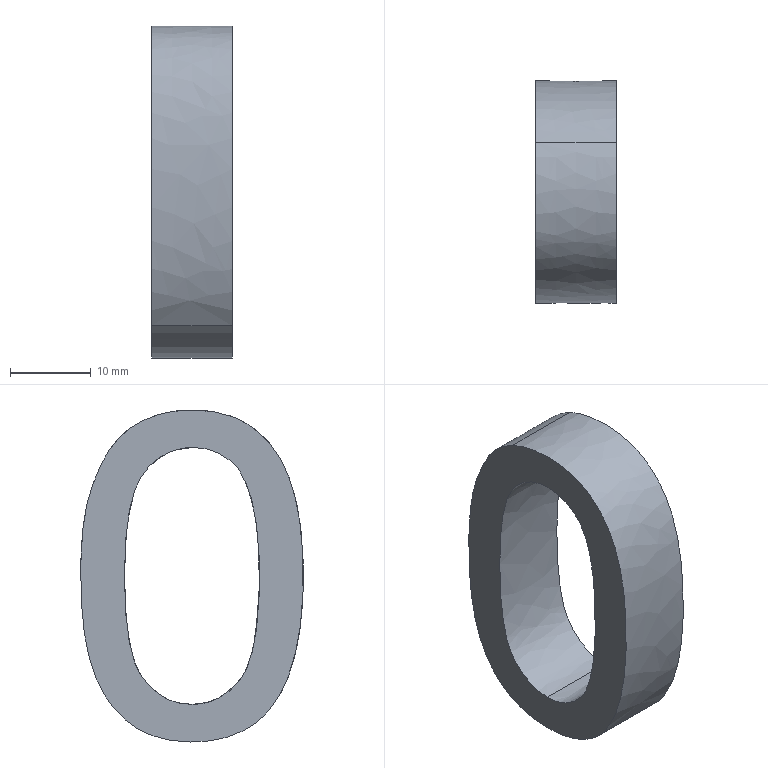Part | NX | features solid 2 | 1 solid | 7 faces | box 10 x 27.595 x 41.147 mm | volume 5024 mm3 | spline 5 | plane 2
STEP:
#1=CARTESIAN_POINT('',(2250.,-393.803,-666.115));
#2=VERTEX_POINT('',#1);
#3=CARTESIAN_POINT('',(2250.,-393.879,-634.268));
#4=VERTEX_POINT('',#3);
#5=CARTESIAN_POINT('',(2250.,-393.803,-666.115));
#6=CARTESIAN_POINT('',(2250.,-391.447,-666.145));
#7=CARTESIAN_POINT('',(2250.,-389.459,-665.12));
#8=CARTESIAN_POINT('',(2250.,-386.216,-661.021));
#9=CARTESIAN_POINT('',(2250.,-385.436,-656.723));
#10=CARTESIAN_POINT('',(2250.,-385.436,-643.843));
#11=CARTESIAN_POINT('',(2250.,-386.216,-639.591));
#12=CARTESIAN_POINT('',(2250.,-387.801,-637.457));
#13=CARTESIAN_POINT('',(2250.,-389.351,-635.369));
#14=CARTESIAN_POINT('',(2250.,-391.401,-634.298));
#15=CARTESIAN_POINT('',(2250.,-393.879,-634.268));
#16=B_SPLINE_CURVE_WITH_KNOTS('',3,(#5,#6,#7,#8,#9,#10,#11,#12,#13,#14,#15),.UNSPECIFIED.,.F.,.F.,(4,2,2,3,4),(0.5149,0.6209,0.7269,0.8299,0.9181),.UNSPECIFIED.);
#17=EDGE_CURVE('',#2,#4,#16,.T.);
#18=ORIENTED_EDGE('',*,*,#17,.F.);
#19=CARTESIAN_POINT('',(2260.,-393.803,-666.115));
#20=VERTEX_POINT('',#19);
#21=CARTESIAN_POINT('',(2260.,-393.803,-666.115));
#22=DIRECTION('',(-1.,0.,0.));
#23=VECTOR('',#22,1000.);
#24=LINE('',#21,#23);
#25=EDGE_CURVE('',#20,#2,#24,.T.);
#26=ORIENTED_EDGE('',*,*,#25,.F.);
#27=CARTESIAN_POINT('',(2260.,-393.879,-634.268));
#28=VERTEX_POINT('',#27);
#29=CARTESIAN_POINT('',(2260.,-393.803,-666.115));
#30=CARTESIAN_POINT('',(2260.,-391.447,-666.145));
#31=CARTESIAN_POINT('',(2260.,-389.459,-665.12));
#32=CARTESIAN_POINT('',(2260.,-386.216,-661.021));
#33=CARTESIAN_POINT('',(2260.,-385.436,-656.723));
#34=CARTESIAN_POINT('',(2260.,-385.436,-643.843));
#35=CARTESIAN_POINT('',(2260.,-386.216,-639.591));
#36=CARTESIAN_POINT('',(2260.,-387.801,-637.457));
#37=CARTESIAN_POINT('',(2260.,-389.351,-635.369));
#38=CARTESIAN_POINT('',(2260.,-391.401,-634.298));
#39=CARTESIAN_POINT('',(2260.,-393.879,-634.268));
#40=B_SPLINE_CURVE_WITH_KNOTS('',3,(#29,#30,#31,#32,#33,#34,#35,#36,#37,#38,#39),.UNSPECIFIED.,.F.,.F.,(4,2,2,3,4),(0.5149,0.6209,0.7269,0.8299,0.9181),.UNSPECIFIED.);
#41=EDGE_CURVE('',#20,#28,#40,.T.);
#42=ORIENTED_EDGE('',*,*,#41,.T.);
#43=CARTESIAN_POINT('',(2260.,-393.879,-634.268));
#44=DIRECTION('',(-1.,0.,0.));
#45=VECTOR('',#44,1000.);
#46=LINE('',#43,#45);
#47=EDGE_CURVE('',#28,#4,#46,.T.);
#48=ORIENTED_EDGE('',*,*,#47,.T.);
#49=EDGE_LOOP('',(#18,#26,#42,#48));
#50=FACE_BOUND('',#49,.T.);
#51=CARTESIAN_POINT('',(2260.,-393.803,-666.115));
#52=CARTESIAN_POINT('',(2250.,-393.803,-666.115));
#53=CARTESIAN_POINT('',(2260.,-392.683,-666.129));
#54=CARTESIAN_POINT('',(2250.,-392.683,-666.129));
#55=CARTESIAN_POINT('',(2260.,-390.613,-665.671));
#56=CARTESIAN_POINT('',(2250.,-390.613,-665.671));
#57=CARTESIAN_POINT('',(2260.,-388.42,-663.972));
#58=CARTESIAN_POINT('',(2250.,-388.42,-663.972));
#59=CARTESIAN_POINT('',(2260.,-386.957,-661.812));
#60=CARTESIAN_POINT('',(2250.,-386.957,-661.812));
#61=CARTESIAN_POINT('',(2260.,-386.173,-659.348));
#62=CARTESIAN_POINT('',(2250.,-386.173,-659.348));
#63=CARTESIAN_POINT('',(2260.,-385.656,-656.143));
#64=CARTESIAN_POINT('',(2250.,-385.656,-656.143));
#65=CARTESIAN_POINT('',(2260.,-385.414,-652.185));
#66=CARTESIAN_POINT('',(2250.,-385.414,-652.185));
#67=CARTESIAN_POINT('',(2260.,-385.436,-647.428));
#68=CARTESIAN_POINT('',(2250.,-385.436,-647.428));
#69=CARTESIAN_POINT('',(2260.,-385.744,-643.63));
#70=CARTESIAN_POINT('',(2250.,-385.744,-643.63));
#71=CARTESIAN_POINT('',(2260.,-386.327,-640.543));
#72=CARTESIAN_POINT('',(2250.,-386.327,-640.543));
#73=CARTESIAN_POINT('',(2260.,-387.073,-638.579));
#74=CARTESIAN_POINT('',(2250.,-387.073,-638.579));
#75=CARTESIAN_POINT('',(2260.,-387.765,-637.464));
#76=CARTESIAN_POINT('',(2250.,-387.765,-637.464));
#77=CARTESIAN_POINT('',(2260.,-388.729,-636.314));
#78=CARTESIAN_POINT('',(2250.,-388.729,-636.314));
#79=CARTESIAN_POINT('',(2260.,-390.537,-634.832));
#80=CARTESIAN_POINT('',(2250.,-390.537,-634.832));
#81=CARTESIAN_POINT('',(2260.,-392.462,-634.285));
#82=CARTESIAN_POINT('',(2250.,-392.462,-634.285));
#83=CARTESIAN_POINT('',(2260.,-393.879,-634.268));
#84=CARTESIAN_POINT('',(2250.,-393.879,-634.268));
#85=B_SPLINE_SURFACE_WITH_KNOTS('',3,1,((#51,#52),(#53,#54),(#55,#56),(#57,#58),(#59,#60),(#61,#62),(#63,#64),(#65,#66),(#67,#68),(#69,#70),(#71,#72),(#73,#74),(#75,#76),(#77,#78),(#79,#80),(#81,#82),(#83,#84)),.SURF_OF_LINEAR_EXTRUSION.,.F.,.F.,.F.,(4,1,1,1,1,1,1,1,1,1,1,1,1,1,4),(2,2),(0.5149,0.5653,0.6157,0.6409,0.6661,0.6913,0.7165,0.7417,0.7669,0.7921,0.8173,0.8299,0.8425,0.8677,0.9181),(0.,1.),.UNSPECIFIED.);
#86=ADVANCED_FACE('',(#50),#85,.T.);
#87=CARTESIAN_POINT('',(2250.,-399.631,-637.067));
#88=VERTEX_POINT('',#87);
#89=CARTESIAN_POINT('',(2250.,-393.879,-634.268));
#90=CARTESIAN_POINT('',(2250.,-396.235,-634.298));
#91=CARTESIAN_POINT('',(2250.,-398.147,-635.216));
#92=CARTESIAN_POINT('',(2250.,-399.631,-637.067));
#93=B_SPLINE_CURVE_WITH_KNOTS('',3,(#89,#90,#91,#92),.UNSPECIFIED.,.F.,.F.,(4,4),(0.9181,1.),.PIECEWISE_BEZIER_KNOTS.);
#94=EDGE_CURVE('',#4,#88,#93,.T.);
#95=ORIENTED_EDGE('',*,*,#94,.F.);
#96=ORIENTED_EDGE('',*,*,#47,.F.);
#97=CARTESIAN_POINT('',(2260.,-399.631,-637.067));
#98=VERTEX_POINT('',#97);
#99=CARTESIAN_POINT('',(2260.,-393.879,-634.268));
#100=CARTESIAN_POINT('',(2260.,-396.235,-634.298));
#101=CARTESIAN_POINT('',(2260.,-398.147,-635.216));
#102=CARTESIAN_POINT('',(2260.,-399.631,-637.067));
#103=B_SPLINE_CURVE_WITH_KNOTS('',3,(#99,#100,#101,#102),.UNSPECIFIED.,.F.,.F.,(4,4),(0.9181,1.),.PIECEWISE_BEZIER_KNOTS.);
#104=EDGE_CURVE('',#28,#98,#103,.T.);
#105=ORIENTED_EDGE('',*,*,#104,.T.);
#106=CARTESIAN_POINT('',(2260.,-399.631,-637.067));
#107=DIRECTION('',(-1.,0.,0.));
#108=VECTOR('',#107,1000.);
#109=LINE('',#106,#108);
#110=EDGE_CURVE('',#98,#88,#109,.T.);
#111=ORIENTED_EDGE('',*,*,#110,.T.);
#112=EDGE_LOOP('',(#95,#96,#105,#111));
#113=FACE_BOUND('',#112,.T.);
#114=CARTESIAN_POINT('',(2260.,-393.879,-634.268));
#115=CARTESIAN_POINT('',(2250.,-393.879,-634.268));
#116=CARTESIAN_POINT('',(2260.,-396.235,-634.298));
#117=CARTESIAN_POINT('',(2250.,-396.235,-634.298));
#118=CARTESIAN_POINT('',(2260.,-398.147,-635.216));
#119=CARTESIAN_POINT('',(2250.,-398.147,-635.216));
#120=CARTESIAN_POINT('',(2260.,-399.631,-637.067));
#121=CARTESIAN_POINT('',(2250.,-399.631,-637.067));
#122=B_SPLINE_SURFACE_WITH_KNOTS('',3,1,((#114,#115),(#116,#117),(#118,#119),(#120,#121)),.SURF_OF_LINEAR_EXTRUSION.,.F.,.F.,.F.,(4,4),(2,2),(0.9181,1.),(0.,1.),.PIECEWISE_BEZIER_KNOTS.);
#123=ADVANCED_FACE('',(#113),#122,.T.);
#124=CARTESIAN_POINT('',(2250.,-403.424,-666.803));
#125=VERTEX_POINT('',#124);
#126=CARTESIAN_POINT('',(2250.,-387.715,-630.948));
#127=VERTEX_POINT('',#126);
#128=CARTESIAN_POINT('',(2250.,-403.424,-666.803));
#129=CARTESIAN_POINT('',(2250.,-406.193,-663.361));
#130=CARTESIAN_POINT('',(2250.,-407.6,-657.824));
#131=CARTESIAN_POINT('',(2250.,-407.6,-645.465));
#132=CARTESIAN_POINT('',(2250.,-407.08,-641.61));
#133=CARTESIAN_POINT('',(2250.,-405.033,-635.653));
#134=CARTESIAN_POINT('',(2250.,-403.501,-633.426));
#135=CARTESIAN_POINT('',(2250.,-401.456,-631.91));
#136=CARTESIAN_POINT('',(2250.,-399.416,-630.398));
#137=CARTESIAN_POINT('',(2250.,-396.893,-629.633));
#138=CARTESIAN_POINT('',(2250.,-393.803,-629.633));
#139=CARTESIAN_POINT('',(2250.,-391.524,-629.633));
#140=CARTESIAN_POINT('',(2250.,-389.489,-630.076));
#141=CARTESIAN_POINT('',(2250.,-387.715,-630.948));
#142=B_SPLINE_CURVE_WITH_KNOTS('',3,(#128,#129,#130,#131,#132,#133,#134,#135,#136,#137,#138,#139,#140,#141),.UNSPECIFIED.,.F.,.F.,(4,2,2,3,3,4),(0.,0.1597,0.2597,0.3593,0.4374,0.4977),.UNSPECIFIED.);
#143=EDGE_CURVE('',#125,#127,#142,.T.);
#144=ORIENTED_EDGE('',*,*,#143,.F.);
#145=CARTESIAN_POINT('',(2260.,-403.424,-666.803));
#146=VERTEX_POINT('',#145);
#147=CARTESIAN_POINT('',(2260.,-403.424,-666.803));
#148=DIRECTION('',(-1.,0.,0.));
#149=VECTOR('',#148,1000.);
#150=LINE('',#147,#149);
#151=EDGE_CURVE('',#146,#125,#150,.T.);
#152=ORIENTED_EDGE('',*,*,#151,.F.);
#153=CARTESIAN_POINT('',(2260.,-387.715,-630.948));
#154=VERTEX_POINT('',#153);
#155=CARTESIAN_POINT('',(2260.,-403.424,-666.803));
#156=CARTESIAN_POINT('',(2260.,-406.193,-663.361));
#157=CARTESIAN_POINT('',(2260.,-407.6,-657.824));
#158=CARTESIAN_POINT('',(2260.,-407.6,-645.465));
#159=CARTESIAN_POINT('',(2260.,-407.08,-641.61));
#160=CARTESIAN_POINT('',(2260.,-405.033,-635.653));
#161=CARTESIAN_POINT('',(2260.,-403.501,-633.426));
#162=CARTESIAN_POINT('',(2260.,-401.456,-631.91));
#163=CARTESIAN_POINT('',(2260.,-399.416,-630.398));
#164=CARTESIAN_POINT('',(2260.,-396.893,-629.633));
#165=CARTESIAN_POINT('',(2260.,-393.803,-629.633));
#166=CARTESIAN_POINT('',(2260.,-391.524,-629.633));
#167=CARTESIAN_POINT('',(2260.,-389.489,-630.076));
#168=CARTESIAN_POINT('',(2260.,-387.715,-630.948));
#169=B_SPLINE_CURVE_WITH_KNOTS('',3,(#155,#156,#157,#158,#159,#160,#161,#162,#163,#164,#165,#166,#167,#168),.UNSPECIFIED.,.F.,.F.,(4,2,2,3,3,4),(0.,0.1597,0.2597,0.3593,0.4374,0.4977),.UNSPECIFIED.);
#170=EDGE_CURVE('',#146,#154,#169,.T.);
#171=ORIENTED_EDGE('',*,*,#170,.T.);
#172=CARTESIAN_POINT('',(2260.,-387.715,-630.948));
#173=DIRECTION('',(-1.,0.,0.));
#174=VECTOR('',#173,1000.);
#175=LINE('',#172,#174);
#176=EDGE_CURVE('',#127,#154,#175,.F.);
#177=ORIENTED_EDGE('',*,*,#176,.F.);
#178=EDGE_LOOP('',(#144,#152,#171,#177));
#179=FACE_BOUND('',#178,.T.);
#180=CARTESIAN_POINT('',(2260.,-403.424,-666.803));
#181=CARTESIAN_POINT('',(2250.,-403.424,-666.803));
#182=CARTESIAN_POINT('',(2260.,-404.503,-665.462));
#183=CARTESIAN_POINT('',(2250.,-404.503,-665.462));
#184=CARTESIAN_POINT('',(2260.,-406.246,-662.143));
#185=CARTESIAN_POINT('',(2250.,-406.246,-662.143));
#186=CARTESIAN_POINT('',(2260.,-407.38,-656.425));
#187=CARTESIAN_POINT('',(2250.,-407.38,-656.425));
#188=CARTESIAN_POINT('',(2260.,-407.616,-651.573));
#189=CARTESIAN_POINT('',(2250.,-407.616,-651.573));
#190=CARTESIAN_POINT('',(2260.,-407.592,-648.603));
#191=CARTESIAN_POINT('',(2250.,-407.592,-648.603));
#192=CARTESIAN_POINT('',(2260.,-407.407,-644.499));
#193=CARTESIAN_POINT('',(2250.,-407.407,-644.499));
#194=CARTESIAN_POINT('',(2260.,-406.568,-639.294));
#195=CARTESIAN_POINT('',(2250.,-406.568,-639.294));
#196=CARTESIAN_POINT('',(2260.,-404.643,-635.165));
#197=CARTESIAN_POINT('',(2250.,-404.643,-635.165));
#198=CARTESIAN_POINT('',(2260.,-402.922,-633.154));
#199=CARTESIAN_POINT('',(2250.,-402.922,-633.154));
#200=CARTESIAN_POINT('',(2260.,-402.015,-632.348));
#201=CARTESIAN_POINT('',(2250.,-402.015,-632.348));
#202=CARTESIAN_POINT('',(2260.,-401.432,-631.875));
#203=CARTESIAN_POINT('',(2250.,-401.432,-631.875));
#204=CARTESIAN_POINT('',(2260.,-400.317,-631.126));
#205=CARTESIAN_POINT('',(2250.,-400.317,-631.126));
#206=CARTESIAN_POINT('',(2260.,-398.954,-630.489));
#207=CARTESIAN_POINT('',(2250.,-398.954,-630.489));
#208=CARTESIAN_POINT('',(2260.,-397.439,-630.01));
#209=CARTESIAN_POINT('',(2250.,-397.439,-630.01));
#210=CARTESIAN_POINT('',(2260.,-395.82,-629.717));
#211=CARTESIAN_POINT('',(2250.,-395.82,-629.717));
#212=CARTESIAN_POINT('',(2260.,-393.408,-629.567));
#213=CARTESIAN_POINT('',(2250.,-393.408,-629.567));
#214=CARTESIAN_POINT('',(2260.,-390.591,-629.828));
#215=CARTESIAN_POINT('',(2250.,-390.591,-629.828));
#216=CARTESIAN_POINT('',(2260.,-388.629,-630.499));
#217=CARTESIAN_POINT('',(2250.,-388.629,-630.499));
#218=CARTESIAN_POINT('',(2260.,-387.715,-630.948));
#219=CARTESIAN_POINT('',(2250.,-387.715,-630.948));
#220=B_SPLINE_SURFACE_WITH_KNOTS('',3,1,((#180,#181),(#182,#183),(#184,#185),(#186,#187),(#188,#189),(#190,#191),(#192,#193),(#194,#195),(#196,#197),(#198,#199),(#200,#201),(#202,#203),(#204,#205),(#206,#207),(#208,#209),(#210,#211),(#212,#213),(#214,#215),(#216,#217),(#218,#219)),.SURF_OF_LINEAR_EXTRUSION.,.F.,.F.,.F.,(4,1,1,1,1,1,1,1,1,1,1,1,1,1,1,1,1,4),(2,2),(0.,0.06221,0.1244,0.1555,0.1711,0.1866,0.2489,0.3111,0.3422,0.35,0.3577,0.3733,0.3888,0.4044,0.4199,0.4355,0.4666,0.4977),(0.,1.),.UNSPECIFIED.);
#221=ADVANCED_FACE('',(#179),#220,.T.);
#222=CARTESIAN_POINT('',(2250.,-387.715,-630.948));
#223=CARTESIAN_POINT('',(2250.,-385.94,-631.82));
#224=CARTESIAN_POINT('',(2250.,-384.518,-633.09));
#225=CARTESIAN_POINT('',(2250.,-382.424,-636.354));
#226=CARTESIAN_POINT('',(2250.,-381.566,-638.382));
#227=CARTESIAN_POINT('',(2250.,-380.296,-643.09));
#228=CARTESIAN_POINT('',(2250.,-380.005,-646.245));
#229=CARTESIAN_POINT('',(2250.,-380.005,-654.979));
#230=CARTESIAN_POINT('',(2250.,-380.495,-658.818));
#231=CARTESIAN_POINT('',(2250.,-381.506,-661.775));
#232=CARTESIAN_POINT('',(2250.,-382.529,-664.769));
#233=CARTESIAN_POINT('',(2250.,-384.074,-667.017));
#234=CARTESIAN_POINT('',(2250.,-388.156,-670.033));
#235=CARTESIAN_POINT('',(2250.,-390.713,-670.78));
#236=CARTESIAN_POINT('',(2250.,-397.887,-670.78));
#237=CARTESIAN_POINT('',(2250.,-401.099,-669.465));
#238=CARTESIAN_POINT('',(2250.,-403.424,-666.803));
#239=B_SPLINE_CURVE_WITH_KNOTS('',3,(#222,#223,#224,#225,#226,#227,#228,#229,#230,#231,#232,#233,#234,#235,#236,#237,#238),.UNSPECIFIED.,.F.,.F.,(4,2,2,2,3,2,2,4),(0.4977,0.5581,0.6192,0.6819,0.7568,0.8304,0.9035,1.),.UNSPECIFIED.);
#240=EDGE_CURVE('',#127,#125,#239,.T.);
#241=ORIENTED_EDGE('',*,*,#240,.F.);
#242=ORIENTED_EDGE('',*,*,#176,.T.);
#243=CARTESIAN_POINT('',(2260.,-387.715,-630.948));
#244=CARTESIAN_POINT('',(2260.,-385.94,-631.82));
#245=CARTESIAN_POINT('',(2260.,-384.518,-633.09));
#246=CARTESIAN_POINT('',(2260.,-382.424,-636.354));
#247=CARTESIAN_POINT('',(2260.,-381.566,-638.382));
#248=CARTESIAN_POINT('',(2260.,-380.296,-643.09));
#249=CARTESIAN_POINT('',(2260.,-380.005,-646.245));
#250=CARTESIAN_POINT('',(2260.,-380.005,-654.979));
#251=CARTESIAN_POINT('',(2260.,-380.495,-658.818));
#252=CARTESIAN_POINT('',(2260.,-381.506,-661.775));
#253=CARTESIAN_POINT('',(2260.,-382.529,-664.769));
#254=CARTESIAN_POINT('',(2260.,-384.074,-667.017));
#255=CARTESIAN_POINT('',(2260.,-388.156,-670.033));
#256=CARTESIAN_POINT('',(2260.,-390.713,-670.78));
#257=CARTESIAN_POINT('',(2260.,-397.887,-670.78));
#258=CARTESIAN_POINT('',(2260.,-401.099,-669.465));
#259=CARTESIAN_POINT('',(2260.,-403.424,-666.803));
#260=B_SPLINE_CURVE_WITH_KNOTS('',3,(#243,#244,#245,#246,#247,#248,#249,#250,#251,#252,#253,#254,#255,#256,#257,#258,#259),.UNSPECIFIED.,.F.,.F.,(4,2,2,2,3,2,2,4),(0.4977,0.5581,0.6192,0.6819,0.7568,0.8304,0.9035,1.),.UNSPECIFIED.);
#261=EDGE_CURVE('',#154,#146,#260,.T.);
#262=ORIENTED_EDGE('',*,*,#261,.T.);
#263=ORIENTED_EDGE('',*,*,#151,.T.);
#264=EDGE_LOOP('',(#241,#242,#262,#263));
#265=FACE_BOUND('',#264,.T.);
#266=CARTESIAN_POINT('',(2260.,-387.715,-630.948));
#267=CARTESIAN_POINT('',(2250.,-387.715,-630.948));
#268=CARTESIAN_POINT('',(2260.,-386.792,-631.402));
#269=CARTESIAN_POINT('',(2250.,-386.792,-631.402));
#270=CARTESIAN_POINT('',(2260.,-385.127,-632.527));
#271=CARTESIAN_POINT('',(2250.,-385.127,-632.527));
#272=CARTESIAN_POINT('',(2260.,-383.28,-634.806));
#273=CARTESIAN_POINT('',(2250.,-383.28,-634.806));
#274=CARTESIAN_POINT('',(2260.,-381.867,-637.71));
#275=CARTESIAN_POINT('',(2250.,-381.867,-637.71));
#276=CARTESIAN_POINT('',(2260.,-380.736,-641.021));
#277=CARTESIAN_POINT('',(2250.,-380.736,-641.021));
#278=CARTESIAN_POINT('',(2260.,-380.199,-644.59));
#279=CARTESIAN_POINT('',(2250.,-380.199,-644.59));
#280=CARTESIAN_POINT('',(2260.,-380.017,-648.051));
#281=CARTESIAN_POINT('',(2250.,-380.017,-648.051));
#282=CARTESIAN_POINT('',(2260.,-379.989,-651.045));
#283=CARTESIAN_POINT('',(2250.,-379.989,-651.045));
#284=CARTESIAN_POINT('',(2260.,-380.087,-653.862));
#285=CARTESIAN_POINT('',(2250.,-380.087,-653.862));
#286=CARTESIAN_POINT('',(2260.,-380.396,-657.281));
#287=CARTESIAN_POINT('',(2250.,-380.396,-657.281));
#288=CARTESIAN_POINT('',(2260.,-381.103,-660.936));
#289=CARTESIAN_POINT('',(2250.,-381.103,-660.936));
#290=CARTESIAN_POINT('',(2260.,-382.547,-664.538));
#291=CARTESIAN_POINT('',(2250.,-382.547,-664.538));
#292=CARTESIAN_POINT('',(2260.,-385.23,-668.305));
#293=CARTESIAN_POINT('',(2250.,-385.23,-668.305));
#294=CARTESIAN_POINT('',(2260.,-388.562,-670.181));
#295=CARTESIAN_POINT('',(2250.,-388.562,-670.181));
#296=CARTESIAN_POINT('',(2260.,-392.128,-670.74));
#297=CARTESIAN_POINT('',(2250.,-392.128,-670.74));
#298=CARTESIAN_POINT('',(2260.,-394.776,-670.837));
#299=CARTESIAN_POINT('',(2250.,-394.776,-670.837));
#300=CARTESIAN_POINT('',(2260.,-399.1,-670.277));
#301=CARTESIAN_POINT('',(2250.,-399.1,-670.277));
#302=CARTESIAN_POINT('',(2260.,-401.912,-668.534));
#303=CARTESIAN_POINT('',(2250.,-401.912,-668.534));
#304=CARTESIAN_POINT('',(2260.,-403.424,-666.803));
#305=CARTESIAN_POINT('',(2250.,-403.424,-666.803));
#306=B_SPLINE_SURFACE_WITH_KNOTS('',3,1,((#266,#267),(#268,#269),(#270,#271),(#272,#273),(#274,#275),(#276,#277),(#278,#279),(#280,#281),(#282,#283),(#284,#285),(#286,#287),(#288,#289),(#290,#291),(#292,#293),(#294,#295),(#296,#297),(#298,#299),(#300,#301),(#302,#303),(#304,#305)),.SURF_OF_LINEAR_EXTRUSION.,.F.,.F.,.F.,(4,1,1,1,1,1,1,1,1,1,1,1,1,1,1,1,1,4),(2,2),(0.4977,0.5291,0.5605,0.5919,0.6233,0.6547,0.6704,0.6861,0.7018,0.7175,0.7489,0.7803,0.8116,0.8744,0.8901,0.9058,0.9372,1.),(0.,1.),.UNSPECIFIED.);
#307=ADVANCED_FACE('',(#265),#306,.T.);
#308=CARTESIAN_POINT('',(2250.,-399.631,-637.067));
#309=CARTESIAN_POINT('',(2250.,-401.298,-639.468));
#310=CARTESIAN_POINT('',(2250.,-402.17,-643.843));
#311=CARTESIAN_POINT('',(2250.,-402.17,-656.753));
#312=CARTESIAN_POINT('',(2250.,-401.359,-661.021));
#313=CARTESIAN_POINT('',(2250.,-399.759,-663.063));
#314=CARTESIAN_POINT('',(2250.,-398.147,-665.12));
#315=CARTESIAN_POINT('',(2250.,-396.158,-666.145));
#316=CARTESIAN_POINT('',(2250.,-393.803,-666.115));
#317=B_SPLINE_CURVE_WITH_KNOTS('',3,(#308,#309,#310,#311,#312,#313,#314,#315,#316),.UNSPECIFIED.,.F.,.F.,(4,2,3,4),(0.,0.201,0.4088,0.5149),.UNSPECIFIED.);
#318=EDGE_CURVE('',#88,#2,#317,.T.);
#319=ORIENTED_EDGE('',*,*,#318,.F.);
#320=ORIENTED_EDGE('',*,*,#110,.F.);
#321=CARTESIAN_POINT('',(2260.,-399.631,-637.067));
#322=CARTESIAN_POINT('',(2260.,-401.298,-639.468));
#323=CARTESIAN_POINT('',(2260.,-402.17,-643.843));
#324=CARTESIAN_POINT('',(2260.,-402.17,-656.753));
#325=CARTESIAN_POINT('',(2260.,-401.359,-661.021));
#326=CARTESIAN_POINT('',(2260.,-399.759,-663.063));
#327=CARTESIAN_POINT('',(2260.,-398.147,-665.12));
#328=CARTESIAN_POINT('',(2260.,-396.158,-666.145));
#329=CARTESIAN_POINT('',(2260.,-393.803,-666.115));
#330=B_SPLINE_CURVE_WITH_KNOTS('',3,(#321,#322,#323,#324,#325,#326,#327,#328,#329),.UNSPECIFIED.,.F.,.F.,(4,2,3,4),(0.,0.201,0.4088,0.5149),.UNSPECIFIED.);
#331=EDGE_CURVE('',#98,#20,#330,.T.);
#332=ORIENTED_EDGE('',*,*,#331,.T.);
#333=ORIENTED_EDGE('',*,*,#25,.T.);
#334=EDGE_LOOP('',(#319,#320,#332,#333));
#335=FACE_BOUND('',#334,.T.);
#336=CARTESIAN_POINT('',(2260.,-399.631,-637.067));
#337=CARTESIAN_POINT('',(2250.,-399.631,-637.067));
#338=CARTESIAN_POINT('',(2260.,-400.164,-637.836));
#339=CARTESIAN_POINT('',(2250.,-400.164,-637.836));
#340=CARTESIAN_POINT('',(2260.,-401.069,-639.777));
#341=CARTESIAN_POINT('',(2250.,-401.069,-639.777));
#342=CARTESIAN_POINT('',(2260.,-401.779,-643.219));
#343=CARTESIAN_POINT('',(2250.,-401.779,-643.219));
#344=CARTESIAN_POINT('',(2260.,-402.088,-646.571));
#345=CARTESIAN_POINT('',(2250.,-402.088,-646.571));
#346=CARTESIAN_POINT('',(2260.,-402.188,-649.411));
#347=CARTESIAN_POINT('',(2250.,-402.188,-649.411));
#348=CARTESIAN_POINT('',(2260.,-402.156,-652.466));
#349=CARTESIAN_POINT('',(2250.,-402.156,-652.466));
#350=CARTESIAN_POINT('',(2260.,-402.01,-655.078));
#351=CARTESIAN_POINT('',(2250.,-402.01,-655.078));
#352=CARTESIAN_POINT('',(2260.,-401.749,-657.393));
#353=CARTESIAN_POINT('',(2250.,-401.749,-657.393));
#354=CARTESIAN_POINT('',(2260.,-401.372,-659.374));
#355=CARTESIAN_POINT('',(2250.,-401.372,-659.374));
#356=CARTESIAN_POINT('',(2260.,-400.88,-661.032));
#357=CARTESIAN_POINT('',(2250.,-400.88,-661.032));
#358=CARTESIAN_POINT('',(2260.,-400.425,-662.035));
#359=CARTESIAN_POINT('',(2250.,-400.425,-662.035));
#360=CARTESIAN_POINT('',(2260.,-400.087,-662.601));
#361=CARTESIAN_POINT('',(2250.,-400.087,-662.601));
#362=CARTESIAN_POINT('',(2260.,-399.908,-662.867));
#363=CARTESIAN_POINT('',(2250.,-399.908,-662.867));
#364=CARTESIAN_POINT('',(2260.,-399.734,-663.102));
#365=CARTESIAN_POINT('',(2250.,-399.734,-663.102));
#366=CARTESIAN_POINT('',(2260.,-399.171,-663.774));
#367=CARTESIAN_POINT('',(2250.,-399.171,-663.774));
#368=CARTESIAN_POINT('',(2260.,-398.543,-664.386));
#369=CARTESIAN_POINT('',(2250.,-398.543,-664.386));
#370=CARTESIAN_POINT('',(2260.,-397.408,-665.251));
#371=CARTESIAN_POINT('',(2250.,-397.408,-665.251));
#372=CARTESIAN_POINT('',(2260.,-395.882,-665.946));
#373=CARTESIAN_POINT('',(2250.,-395.882,-665.946));
#374=CARTESIAN_POINT('',(2260.,-394.518,-666.124));
#375=CARTESIAN_POINT('',(2250.,-394.518,-666.124));
#376=CARTESIAN_POINT('',(2260.,-393.803,-666.115));
#377=CARTESIAN_POINT('',(2250.,-393.803,-666.115));
#378=B_SPLINE_SURFACE_WITH_KNOTS('',3,1,((#336,#337),(#338,#339),(#340,#341),(#342,#343),(#344,#345),(#346,#347),(#348,#349),(#350,#351),(#352,#353),(#354,#355),(#356,#357),(#358,#359),(#360,#361),(#362,#363),(#364,#365),(#366,#367),(#368,#369),(#370,#371),(#372,#373),(#374,#375),(#376,#377)),.SURF_OF_LINEAR_EXTRUSION.,.F.,.F.,.F.,(4,1,1,1,1,1,1,1,1,1,1,1,1,1,1,1,1,1,4),(2,2),(0.,0.06436,0.1287,0.1609,0.1931,0.2253,0.2574,0.2896,0.3218,0.354,0.3861,0.3942,0.4022,0.4103,0.4183,0.4344,0.4505,0.4827,0.5149),(0.,1.),.UNSPECIFIED.);
#379=ADVANCED_FACE('',(#335),#378,.T.);
#380=ORIENTED_EDGE('',*,*,#170,.F.);
#381=ORIENTED_EDGE('',*,*,#261,.F.);
#382=EDGE_LOOP('',(#380,#381));
#383=FACE_BOUND('',#382,.T.);
#384=ORIENTED_EDGE('',*,*,#41,.F.);
#385=ORIENTED_EDGE('',*,*,#331,.F.);
#386=ORIENTED_EDGE('',*,*,#104,.F.);
#387=EDGE_LOOP('',(#384,#385,#386));
#388=FACE_BOUND('',#387,.T.);
#389=CARTESIAN_POINT('',(2260.,-406.37,-639.625));
#390=DIRECTION('',(1.,0.,0.));
#391=DIRECTION('',(0.,1.,0.));
#392=AXIS2_PLACEMENT_3D('',#389,#390,#391);
#393=PLANE('',#392);
#394=ADVANCED_FACE('',(#383,#388),#393,.T.);
#395=ORIENTED_EDGE('',*,*,#143,.T.);
#396=ORIENTED_EDGE('',*,*,#240,.T.);
#397=EDGE_LOOP('',(#395,#396));
#398=FACE_BOUND('',#397,.T.);
#399=ORIENTED_EDGE('',*,*,#17,.T.);
#400=ORIENTED_EDGE('',*,*,#94,.T.);
#401=ORIENTED_EDGE('',*,*,#318,.T.);
#402=EDGE_LOOP('',(#399,#400,#401));
#403=FACE_BOUND('',#402,.T.);
#404=CARTESIAN_POINT('',(2250.,-406.37,-639.625));
#405=DIRECTION('',(1.,0.,0.));
#406=DIRECTION('',(0.,1.,0.));
#407=AXIS2_PLACEMENT_3D('',#404,#405,#406);
#408=PLANE('',#407);
#409=ADVANCED_FACE('',(#398,#403),#408,.F.);
#410=CLOSED_SHELL('',(#86,#123,#221,#307,#379,#394,#409));
#411=MANIFOLD_SOLID_BREP('',#410);
#412=(LENGTH_UNIT()NAMED_UNIT(*)SI_UNIT(.MILLI.,.METRE.));
#413=UNCERTAINTY_MEASURE_WITH_UNIT(LENGTH_MEASURE(0.0508),#412,'','');
#414=(NAMED_UNIT(*)PLANE_ANGLE_UNIT()SI_UNIT($,.RADIAN.));
#415=(NAMED_UNIT(*)SI_UNIT($,.STERADIAN.)SOLID_ANGLE_UNIT());
#416=(GEOMETRIC_REPRESENTATION_CONTEXT(3)GLOBAL_UNCERTAINTY_ASSIGNED_CONTEXT((#413))GLOBAL_UNIT_ASSIGNED_CONTEXT((#412,#414,#415))REPRESENTATION_CONTEXT('',''));
#417=ADVANCED_BREP_SHAPE_REPRESENTATION('',(#411),#416);